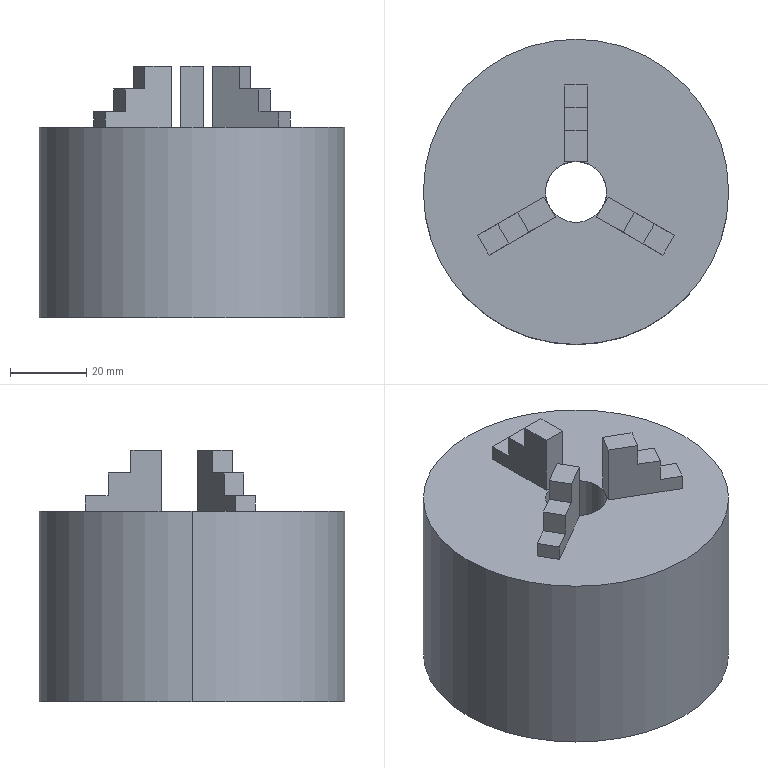Part | SolidWorks | features ICE 4, CirPattern 2, Extrusion 1, HoleWzd 1 | 1 solid | 45 faces | box 80 x 80 x 66 mm | volume 244059 mm3 | plane 29 | cylinder 10 | cone 6 | commonest cylinder face diameters 5 x6 16 x2 80 x2
STEP:
#1=CARTESIAN_POINT('',(-26.079,-16.5,17.));
#2=VERTEX_POINT('',#1);
#3=CARTESIAN_POINT('',(-31.079,-16.5,17.));
#4=VERTEX_POINT('',#3);
#5=CARTESIAN_POINT('',(-28.579,-16.5,17.));
#6=DIRECTION('',(0.,0.,-1.));
#7=DIRECTION('',(-1.,0.,0.));
#8=AXIS2_PLACEMENT_3D('',#5,#6,#7);
#9=CIRCLE('',#8,2.5);
#10=EDGE_CURVE('',#2,#4,#9,.T.);
#11=ORIENTED_EDGE('',*,*,#10,.F.);
#12=CARTESIAN_POINT('',(-26.079,-16.5,0.));
#13=VERTEX_POINT('',#12);
#14=CARTESIAN_POINT('',(-26.079,-16.5,0.));
#15=DIRECTION('',(0.,0.,-1.));
#16=VECTOR('',#15,1000.);
#17=LINE('',#14,#16);
#18=EDGE_CURVE('',#2,#13,#17,.T.);
#19=ORIENTED_EDGE('',*,*,#18,.T.);
#20=CARTESIAN_POINT('',(-31.079,-16.5,0.));
#21=VERTEX_POINT('',#20);
#22=CARTESIAN_POINT('',(-28.579,-16.5,0.));
#23=DIRECTION('',(0.,0.,-1.));
#24=DIRECTION('',(-1.,0.,0.));
#25=AXIS2_PLACEMENT_3D('',#22,#23,#24);
#26=CIRCLE('',#25,2.5);
#27=EDGE_CURVE('',#13,#21,#26,.T.);
#28=ORIENTED_EDGE('',*,*,#27,.T.);
#29=CARTESIAN_POINT('',(-31.079,-16.5,0.));
#30=DIRECTION('',(0.,0.,-1.));
#31=VECTOR('',#30,1000.);
#32=LINE('',#29,#31);
#33=EDGE_CURVE('',#4,#21,#32,.T.);
#34=ORIENTED_EDGE('',*,*,#33,.F.);
#35=EDGE_LOOP('',(#11,#19,#28,#34));
#36=FACE_OUTER_BOUND('',#35,.T.);
#37=CARTESIAN_POINT('',(-28.579,-16.5,0.));
#38=DIRECTION('',(0.,0.,-1.));
#39=DIRECTION('',(-1.,0.,0.));
#40=AXIS2_PLACEMENT_3D('',#37,#38,#39);
#41=CYLINDRICAL_SURFACE('',#40,2.5);
#42=ADVANCED_FACE('',(#36),#41,.F.);
#43=CARTESIAN_POINT('',(-28.579,-16.5,18.502));
#44=VERTEX_POINT('',#43);
#45=CARTESIAN_POINT('',(-31.079,-16.5,17.));
#46=DIRECTION('',(-0.8572,0.,-0.515));
#47=VECTOR('',#46,1000.);
#48=LINE('',#45,#47);
#49=EDGE_CURVE('',#44,#4,#48,.T.);
#50=ORIENTED_EDGE('',*,*,#49,.F.);
#51=CARTESIAN_POINT('',(-26.079,-16.5,17.));
#52=DIRECTION('',(0.8572,0.,-0.515));
#53=VECTOR('',#52,1000.);
#54=LINE('',#51,#53);
#55=EDGE_CURVE('',#44,#2,#54,.T.);
#56=ORIENTED_EDGE('',*,*,#55,.T.);
#57=ORIENTED_EDGE('',*,*,#10,.T.);
#58=EDGE_LOOP('',(#50,#56,#57));
#59=FACE_OUTER_BOUND('',#58,.T.);
#60=CARTESIAN_POINT('',(-28.579,-16.5,17.));
#61=DIRECTION('',(0.,0.,-1.));
#62=DIRECTION('',(-1.,0.,0.));
#63=AXIS2_PLACEMENT_3D('',#60,#61,#62);
#64=CONICAL_SURFACE('',#63,2.5,1.03);
#65=ADVANCED_FACE('',(#59),#64,.F.);
#66=CARTESIAN_POINT('',(31.079,-16.5,17.));
#67=VERTEX_POINT('',#66);
#68=CARTESIAN_POINT('',(26.079,-16.5,17.));
#69=VERTEX_POINT('',#68);
#70=CARTESIAN_POINT('',(28.579,-16.5,17.));
#71=DIRECTION('',(0.,0.,-1.));
#72=DIRECTION('',(-1.,0.,0.));
#73=AXIS2_PLACEMENT_3D('',#70,#71,#72);
#74=CIRCLE('',#73,2.5);
#75=EDGE_CURVE('',#67,#69,#74,.T.);
#76=ORIENTED_EDGE('',*,*,#75,.F.);
#77=CARTESIAN_POINT('',(31.079,-16.5,0.));
#78=VERTEX_POINT('',#77);
#79=CARTESIAN_POINT('',(31.079,-16.5,0.));
#80=DIRECTION('',(0.,0.,-1.));
#81=VECTOR('',#80,1000.);
#82=LINE('',#79,#81);
#83=EDGE_CURVE('',#67,#78,#82,.T.);
#84=ORIENTED_EDGE('',*,*,#83,.T.);
#85=CARTESIAN_POINT('',(26.079,-16.5,0.));
#86=VERTEX_POINT('',#85);
#87=CARTESIAN_POINT('',(28.579,-16.5,0.));
#88=DIRECTION('',(0.,0.,-1.));
#89=DIRECTION('',(-1.,0.,0.));
#90=AXIS2_PLACEMENT_3D('',#87,#88,#89);
#91=CIRCLE('',#90,2.5);
#92=EDGE_CURVE('',#78,#86,#91,.T.);
#93=ORIENTED_EDGE('',*,*,#92,.T.);
#94=CARTESIAN_POINT('',(26.079,-16.5,0.));
#95=DIRECTION('',(0.,0.,-1.));
#96=VECTOR('',#95,1000.);
#97=LINE('',#94,#96);
#98=EDGE_CURVE('',#69,#86,#97,.T.);
#99=ORIENTED_EDGE('',*,*,#98,.F.);
#100=EDGE_LOOP('',(#76,#84,#93,#99));
#101=FACE_OUTER_BOUND('',#100,.T.);
#102=CARTESIAN_POINT('',(28.579,-16.5,0.));
#103=DIRECTION('',(0.,0.,-1.));
#104=DIRECTION('',(-1.,0.,0.));
#105=AXIS2_PLACEMENT_3D('',#102,#103,#104);
#106=CYLINDRICAL_SURFACE('',#105,2.5);
#107=ADVANCED_FACE('',(#101),#106,.F.);
#108=CARTESIAN_POINT('',(28.579,-16.5,18.502));
#109=VERTEX_POINT('',#108);
#110=CARTESIAN_POINT('',(26.079,-16.5,17.));
#111=DIRECTION('',(-0.8572,0.,-0.515));
#112=VECTOR('',#111,1000.);
#113=LINE('',#110,#112);
#114=EDGE_CURVE('',#109,#69,#113,.T.);
#115=ORIENTED_EDGE('',*,*,#114,.F.);
#116=CARTESIAN_POINT('',(31.079,-16.5,17.));
#117=DIRECTION('',(0.8572,0.,-0.515));
#118=VECTOR('',#117,1000.);
#119=LINE('',#116,#118);
#120=EDGE_CURVE('',#109,#67,#119,.T.);
#121=ORIENTED_EDGE('',*,*,#120,.T.);
#122=ORIENTED_EDGE('',*,*,#75,.T.);
#123=EDGE_LOOP('',(#115,#121,#122));
#124=FACE_OUTER_BOUND('',#123,.T.);
#125=CARTESIAN_POINT('',(28.579,-16.5,17.));
#126=DIRECTION('',(0.,0.,-1.));
#127=DIRECTION('',(-1.,0.,0.));
#128=AXIS2_PLACEMENT_3D('',#125,#126,#127);
#129=CONICAL_SURFACE('',#128,2.5,1.03);
#130=ADVANCED_FACE('',(#124),#129,.F.);
#131=CARTESIAN_POINT('',(2.5,33.,17.));
#132=VERTEX_POINT('',#131);
#133=CARTESIAN_POINT('',(-2.5,33.,17.));
#134=VERTEX_POINT('',#133);
#135=CARTESIAN_POINT('',(0.,33.,17.));
#136=DIRECTION('',(0.,0.,-1.));
#137=DIRECTION('',(-1.,0.,0.));
#138=AXIS2_PLACEMENT_3D('',#135,#136,#137);
#139=CIRCLE('',#138,2.5);
#140=EDGE_CURVE('',#132,#134,#139,.T.);
#141=ORIENTED_EDGE('',*,*,#140,.F.);
#142=CARTESIAN_POINT('',(2.5,33.,0.));
#143=VERTEX_POINT('',#142);
#144=CARTESIAN_POINT('',(2.5,33.,0.));
#145=DIRECTION('',(0.,0.,-1.));
#146=VECTOR('',#145,1000.);
#147=LINE('',#144,#146);
#148=EDGE_CURVE('',#132,#143,#147,.T.);
#149=ORIENTED_EDGE('',*,*,#148,.T.);
#150=CARTESIAN_POINT('',(-2.5,33.,0.));
#151=VERTEX_POINT('',#150);
#152=CARTESIAN_POINT('',(0.,33.,0.));
#153=DIRECTION('',(0.,0.,-1.));
#154=DIRECTION('',(-1.,0.,0.));
#155=AXIS2_PLACEMENT_3D('',#152,#153,#154);
#156=CIRCLE('',#155,2.5);
#157=EDGE_CURVE('',#143,#151,#156,.T.);
#158=ORIENTED_EDGE('',*,*,#157,.T.);
#159=CARTESIAN_POINT('',(-2.5,33.,0.));
#160=DIRECTION('',(0.,0.,-1.));
#161=VECTOR('',#160,1000.);
#162=LINE('',#159,#161);
#163=EDGE_CURVE('',#134,#151,#162,.T.);
#164=ORIENTED_EDGE('',*,*,#163,.F.);
#165=EDGE_LOOP('',(#141,#149,#158,#164));
#166=FACE_OUTER_BOUND('',#165,.T.);
#167=CARTESIAN_POINT('',(0.,33.,0.));
#168=DIRECTION('',(0.,0.,-1.));
#169=DIRECTION('',(-1.,0.,0.));
#170=AXIS2_PLACEMENT_3D('',#167,#168,#169);
#171=CYLINDRICAL_SURFACE('',#170,2.5);
#172=ADVANCED_FACE('',(#166),#171,.F.);
#173=CARTESIAN_POINT('',(0.,33.,18.502));
#174=VERTEX_POINT('',#173);
#175=CARTESIAN_POINT('',(-2.5,33.,17.));
#176=DIRECTION('',(-0.8572,0.,-0.515));
#177=VECTOR('',#176,1000.);
#178=LINE('',#175,#177);
#179=EDGE_CURVE('',#174,#134,#178,.T.);
#180=ORIENTED_EDGE('',*,*,#179,.F.);
#181=CARTESIAN_POINT('',(2.5,33.,17.));
#182=DIRECTION('',(0.8572,0.,-0.515));
#183=VECTOR('',#182,1000.);
#184=LINE('',#181,#183);
#185=EDGE_CURVE('',#174,#132,#184,.T.);
#186=ORIENTED_EDGE('',*,*,#185,.T.);
#187=ORIENTED_EDGE('',*,*,#140,.T.);
#188=EDGE_LOOP('',(#180,#186,#187));
#189=FACE_OUTER_BOUND('',#188,.T.);
#190=CARTESIAN_POINT('',(0.,33.,17.));
#191=DIRECTION('',(0.,0.,-1.));
#192=DIRECTION('',(-1.,0.,0.));
#193=AXIS2_PLACEMENT_3D('',#190,#191,#192);
#194=CONICAL_SURFACE('',#193,2.5,1.03);
#195=ADVANCED_FACE('',(#189),#194,.F.);
#196=CARTESIAN_POINT('',(6.928,-4.,50.));
#197=VERTEX_POINT('',#196);
#198=CARTESIAN_POINT('',(8.,0.,50.));
#199=VERTEX_POINT('',#198);
#200=CARTESIAN_POINT('',(0.,0.,50.));
#201=DIRECTION('',(0.,0.,1.));
#202=DIRECTION('',(1.,0.,0.));
#203=AXIS2_PLACEMENT_3D('',#200,#201,#202);
#204=CIRCLE('',#203,8.);
#205=EDGE_CURVE('',#197,#199,#204,.T.);
#206=ORIENTED_EDGE('',*,*,#205,.T.);
#207=CARTESIAN_POINT('',(8.,0.,0.));
#208=VERTEX_POINT('',#207);
#209=CARTESIAN_POINT('',(8.,0.,66.));
#210=DIRECTION('',(0.,0.,-1.));
#211=VECTOR('',#210,1000.);
#212=LINE('',#209,#211);
#213=EDGE_CURVE('',#199,#208,#212,.T.);
#214=ORIENTED_EDGE('',*,*,#213,.T.);
#215=CARTESIAN_POINT('',(-8.,0.,0.));
#216=VERTEX_POINT('',#215);
#217=CARTESIAN_POINT('',(0.,0.,0.));
#218=DIRECTION('',(0.,0.,-1.));
#219=DIRECTION('',(-1.,0.,0.));
#220=AXIS2_PLACEMENT_3D('',#217,#218,#219);
#221=CIRCLE('',#220,8.);
#222=EDGE_CURVE('',#208,#216,#221,.T.);
#223=ORIENTED_EDGE('',*,*,#222,.T.);
#224=CARTESIAN_POINT('',(-8.,0.,50.));
#225=VERTEX_POINT('',#224);
#226=CARTESIAN_POINT('',(-8.,0.,66.));
#227=DIRECTION('',(0.,0.,-1.));
#228=VECTOR('',#227,1000.);
#229=LINE('',#226,#228);
#230=EDGE_CURVE('',#225,#216,#229,.T.);
#231=ORIENTED_EDGE('',*,*,#230,.F.);
#232=CARTESIAN_POINT('',(-6.928,-4.,50.));
#233=VERTEX_POINT('',#232);
#234=CARTESIAN_POINT('',(0.,0.,50.));
#235=DIRECTION('',(0.,0.,1.));
#236=DIRECTION('',(1.,0.,0.));
#237=AXIS2_PLACEMENT_3D('',#234,#235,#236);
#238=CIRCLE('',#237,8.);
#239=EDGE_CURVE('',#225,#233,#238,.T.);
#240=ORIENTED_EDGE('',*,*,#239,.T.);
#241=CARTESIAN_POINT('',(0.,0.,50.));
#242=DIRECTION('',(0.,0.,1.));
#243=DIRECTION('',(1.,0.,0.));
#244=AXIS2_PLACEMENT_3D('',#241,#242,#243);
#245=CIRCLE('',#244,8.);
#246=EDGE_CURVE('',#233,#197,#245,.T.);
#247=ORIENTED_EDGE('',*,*,#246,.T.);
#248=EDGE_LOOP('',(#206,#214,#223,#231,#240,#247));
#249=FACE_OUTER_BOUND('',#248,.T.);
#250=CARTESIAN_POINT('',(0.,0.,66.));
#251=DIRECTION('',(0.,0.,-1.));
#252=DIRECTION('',(-1.,0.,0.));
#253=AXIS2_PLACEMENT_3D('',#250,#251,#252);
#254=CYLINDRICAL_SURFACE('',#253,8.);
#255=ADVANCED_FACE('',(#249),#254,.F.);
#256=CARTESIAN_POINT('',(40.,0.,50.));
#257=VERTEX_POINT('',#256);
#258=CARTESIAN_POINT('',(-40.,0.,50.));
#259=VERTEX_POINT('',#258);
#260=CARTESIAN_POINT('',(0.,0.,50.));
#261=DIRECTION('',(0.,0.,1.));
#262=DIRECTION('',(1.,0.,0.));
#263=AXIS2_PLACEMENT_3D('',#260,#261,#262);
#264=CIRCLE('',#263,40.);
#265=EDGE_CURVE('',#257,#259,#264,.T.);
#266=ORIENTED_EDGE('',*,*,#265,.F.);
#267=CARTESIAN_POINT('',(40.,0.,0.));
#268=VERTEX_POINT('',#267);
#269=CARTESIAN_POINT('',(40.,0.,50.));
#270=DIRECTION('',(0.,0.,-1.));
#271=VECTOR('',#270,1000.);
#272=LINE('',#269,#271);
#273=EDGE_CURVE('',#257,#268,#272,.T.);
#274=ORIENTED_EDGE('',*,*,#273,.T.);
#275=CARTESIAN_POINT('',(-40.,0.,0.));
#276=VERTEX_POINT('',#275);
#277=CARTESIAN_POINT('',(0.,0.,0.));
#278=DIRECTION('',(0.,0.,1.));
#279=DIRECTION('',(1.,0.,0.));
#280=AXIS2_PLACEMENT_3D('',#277,#278,#279);
#281=CIRCLE('',#280,40.);
#282=EDGE_CURVE('',#268,#276,#281,.T.);
#283=ORIENTED_EDGE('',*,*,#282,.T.);
#284=CARTESIAN_POINT('',(-40.,0.,50.));
#285=DIRECTION('',(0.,0.,-1.));
#286=VECTOR('',#285,1000.);
#287=LINE('',#284,#286);
#288=EDGE_CURVE('',#259,#276,#287,.T.);
#289=ORIENTED_EDGE('',*,*,#288,.F.);
#290=EDGE_LOOP('',(#266,#274,#283,#289));
#291=FACE_OUTER_BOUND('',#290,.T.);
#292=CARTESIAN_POINT('',(0.,0.,50.));
#293=DIRECTION('',(0.,0.,-1.));
#294=DIRECTION('',(-1.,0.,0.));
#295=AXIS2_PLACEMENT_3D('',#292,#293,#294);
#296=CYLINDRICAL_SURFACE('',#295,40.);
#297=ADVANCED_FACE('',(#291),#296,.T.);
#298=CARTESIAN_POINT('',(0.,8.,50.));
#299=VERTEX_POINT('',#298);
#300=CARTESIAN_POINT('',(0.,0.,50.));
#301=DIRECTION('',(0.,0.,1.));
#302=DIRECTION('',(1.,0.,0.));
#303=AXIS2_PLACEMENT_3D('',#300,#301,#302);
#304=CIRCLE('',#303,8.);
#305=EDGE_CURVE('',#299,#225,#304,.T.);
#306=ORIENTED_EDGE('',*,*,#305,.F.);
#307=CARTESIAN_POINT('',(-3.,8.,50.));
#308=VERTEX_POINT('',#307);
#309=CARTESIAN_POINT('',(-3.,8.,50.));
#310=DIRECTION('',(1.,0.,0.));
#311=VECTOR('',#310,1000.);
#312=LINE('',#309,#311);
#313=EDGE_CURVE('',#308,#299,#312,.T.);
#314=ORIENTED_EDGE('',*,*,#313,.F.);
#315=CARTESIAN_POINT('',(-3.,28.,50.));
#316=VERTEX_POINT('',#315);
#317=CARTESIAN_POINT('',(-3.,8.,50.));
#318=DIRECTION('',(0.,-1.,0.));
#319=VECTOR('',#318,1000.);
#320=LINE('',#317,#319);
#321=EDGE_CURVE('',#316,#308,#320,.T.);
#322=ORIENTED_EDGE('',*,*,#321,.F.);
#323=CARTESIAN_POINT('',(3.,28.,50.));
#324=VERTEX_POINT('',#323);
#325=CARTESIAN_POINT('',(-3.,28.,50.));
#326=DIRECTION('',(-1.,0.,0.));
#327=VECTOR('',#326,1000.);
#328=LINE('',#325,#327);
#329=EDGE_CURVE('',#324,#316,#328,.T.);
#330=ORIENTED_EDGE('',*,*,#329,.F.);
#331=CARTESIAN_POINT('',(3.,8.,50.));
#332=VERTEX_POINT('',#331);
#333=CARTESIAN_POINT('',(3.,8.,50.));
#334=DIRECTION('',(0.,1.,0.));
#335=VECTOR('',#334,1000.);
#336=LINE('',#333,#335);
#337=EDGE_CURVE('',#332,#324,#336,.T.);
#338=ORIENTED_EDGE('',*,*,#337,.F.);
#339=CARTESIAN_POINT('',(-3.,8.,50.));
#340=DIRECTION('',(1.,0.,0.));
#341=VECTOR('',#340,1000.);
#342=LINE('',#339,#341);
#343=EDGE_CURVE('',#299,#332,#342,.T.);
#344=ORIENTED_EDGE('',*,*,#343,.F.);
#345=CARTESIAN_POINT('',(0.,0.,50.));
#346=DIRECTION('',(0.,0.,1.));
#347=DIRECTION('',(1.,0.,0.));
#348=AXIS2_PLACEMENT_3D('',#345,#346,#347);
#349=CIRCLE('',#348,8.);
#350=EDGE_CURVE('',#199,#299,#349,.T.);
#351=ORIENTED_EDGE('',*,*,#350,.F.);
#352=ORIENTED_EDGE('',*,*,#205,.F.);
#353=CARTESIAN_POINT('',(8.428,-1.402,50.));
#354=VERTEX_POINT('',#353);
#355=CARTESIAN_POINT('',(8.428,-1.402,50.));
#356=DIRECTION('',(-0.5,-0.866,0.));
#357=VECTOR('',#356,1000.);
#358=LINE('',#355,#357);
#359=EDGE_CURVE('',#354,#197,#358,.T.);
#360=ORIENTED_EDGE('',*,*,#359,.F.);
#361=CARTESIAN_POINT('',(25.749,-11.402,50.));
#362=VERTEX_POINT('',#361);
#363=CARTESIAN_POINT('',(8.428,-1.402,50.));
#364=DIRECTION('',(-0.866,0.5,0.));
#365=VECTOR('',#364,1000.);
#366=LINE('',#363,#365);
#367=EDGE_CURVE('',#362,#354,#366,.T.);
#368=ORIENTED_EDGE('',*,*,#367,.F.);
#369=CARTESIAN_POINT('',(22.749,-16.598,50.));
#370=VERTEX_POINT('',#369);
#371=CARTESIAN_POINT('',(25.749,-11.402,50.));
#372=DIRECTION('',(0.5,0.866,0.));
#373=VECTOR('',#372,1000.);
#374=LINE('',#371,#373);
#375=EDGE_CURVE('',#370,#362,#374,.T.);
#376=ORIENTED_EDGE('',*,*,#375,.F.);
#377=CARTESIAN_POINT('',(5.428,-6.598,50.));
#378=VERTEX_POINT('',#377);
#379=CARTESIAN_POINT('',(5.428,-6.598,50.));
#380=DIRECTION('',(0.866,-0.5,0.));
#381=VECTOR('',#380,1000.);
#382=LINE('',#379,#381);
#383=EDGE_CURVE('',#378,#370,#382,.T.);
#384=ORIENTED_EDGE('',*,*,#383,.F.);
#385=CARTESIAN_POINT('',(8.428,-1.402,50.));
#386=DIRECTION('',(-0.5,-0.866,0.));
#387=VECTOR('',#386,1000.);
#388=LINE('',#385,#387);
#389=EDGE_CURVE('',#197,#378,#388,.T.);
#390=ORIENTED_EDGE('',*,*,#389,.F.);
#391=ORIENTED_EDGE('',*,*,#246,.F.);
#392=CARTESIAN_POINT('',(-5.428,-6.598,50.));
#393=VERTEX_POINT('',#392);
#394=CARTESIAN_POINT('',(-5.428,-6.598,50.));
#395=DIRECTION('',(-0.5,0.866,0.));
#396=VECTOR('',#395,1000.);
#397=LINE('',#394,#396);
#398=EDGE_CURVE('',#393,#233,#397,.T.);
#399=ORIENTED_EDGE('',*,*,#398,.F.);
#400=CARTESIAN_POINT('',(-22.749,-16.598,50.));
#401=VERTEX_POINT('',#400);
#402=CARTESIAN_POINT('',(-5.428,-6.598,50.));
#403=DIRECTION('',(0.866,0.5,0.));
#404=VECTOR('',#403,1000.);
#405=LINE('',#402,#404);
#406=EDGE_CURVE('',#401,#393,#405,.T.);
#407=ORIENTED_EDGE('',*,*,#406,.F.);
#408=CARTESIAN_POINT('',(-25.749,-11.402,50.));
#409=VERTEX_POINT('',#408);
#410=CARTESIAN_POINT('',(-22.749,-16.598,50.));
#411=DIRECTION('',(0.5,-0.866,0.));
#412=VECTOR('',#411,1000.);
#413=LINE('',#410,#412);
#414=EDGE_CURVE('',#409,#401,#413,.T.);
#415=ORIENTED_EDGE('',*,*,#414,.F.);
#416=CARTESIAN_POINT('',(-8.428,-1.402,50.));
#417=VERTEX_POINT('',#416);
#418=CARTESIAN_POINT('',(-8.428,-1.402,50.));
#419=DIRECTION('',(-0.866,-0.5,0.));
#420=VECTOR('',#419,1000.);
#421=LINE('',#418,#420);
#422=EDGE_CURVE('',#417,#409,#421,.T.);
#423=ORIENTED_EDGE('',*,*,#422,.F.);
#424=CARTESIAN_POINT('',(-5.428,-6.598,50.));
#425=DIRECTION('',(-0.5,0.866,0.));
#426=VECTOR('',#425,1000.);
#427=LINE('',#424,#426);
#428=EDGE_CURVE('',#233,#417,#427,.T.);
#429=ORIENTED_EDGE('',*,*,#428,.F.);
#430=ORIENTED_EDGE('',*,*,#239,.F.);
#431=EDGE_LOOP('',(#306,#314,#322,#330,#338,#344,#351,#352,#360,#368,#376,#384,#390,#391,#399,#407,#415,#423,#429,#430));
#432=FACE_BOUND('',#431,.T.);
#433=CARTESIAN_POINT('',(0.,0.,50.));
#434=DIRECTION('',(0.,0.,1.));
#435=DIRECTION('',(1.,0.,0.));
#436=AXIS2_PLACEMENT_3D('',#433,#434,#435);
#437=CIRCLE('',#436,40.);
#438=EDGE_CURVE('',#259,#257,#437,.T.);
#439=ORIENTED_EDGE('',*,*,#438,.T.);
#440=ORIENTED_EDGE('',*,*,#265,.T.);
#441=EDGE_LOOP('',(#439,#440));
#442=FACE_OUTER_BOUND('',#441,.T.);
#443=CARTESIAN_POINT('',(0.,0.,50.));
#444=DIRECTION('',(0.,0.,1.));
#445=DIRECTION('',(1.,0.,0.));
#446=AXIS2_PLACEMENT_3D('',#443,#444,#445);
#447=PLANE('',#446);
#448=ADVANCED_FACE('',(#432,#442),#447,.T.);
#449=ORIENTED_EDGE('',*,*,#273,.F.);
#450=ORIENTED_EDGE('',*,*,#438,.F.);
#451=ORIENTED_EDGE('',*,*,#288,.T.);
#452=CARTESIAN_POINT('',(0.,0.,0.));
#453=DIRECTION('',(0.,0.,1.));
#454=DIRECTION('',(1.,0.,0.));
#455=AXIS2_PLACEMENT_3D('',#452,#453,#454);
#456=CIRCLE('',#455,40.);
#457=EDGE_CURVE('',#276,#268,#456,.T.);
#458=ORIENTED_EDGE('',*,*,#457,.T.);
#459=EDGE_LOOP('',(#449,#450,#451,#458));
#460=FACE_OUTER_BOUND('',#459,.T.);
#461=CARTESIAN_POINT('',(0.,0.,50.));
#462=DIRECTION('',(0.,0.,-1.));
#463=DIRECTION('',(-1.,0.,0.));
#464=AXIS2_PLACEMENT_3D('',#461,#462,#463);
#465=CYLINDRICAL_SURFACE('',#464,40.);
#466=ADVANCED_FACE('',(#460),#465,.T.);
#467=CARTESIAN_POINT('',(-28.579,-16.5,0.));
#468=DIRECTION('',(0.,0.,-1.));
#469=DIRECTION('',(-1.,0.,0.));
#470=AXIS2_PLACEMENT_3D('',#467,#468,#469);
#471=CIRCLE('',#470,2.5);
#472=EDGE_CURVE('',#21,#13,#471,.T.);
#473=ORIENTED_EDGE('',*,*,#472,.F.);
#474=ORIENTED_EDGE('',*,*,#27,.F.);
#475=EDGE_LOOP('',(#473,#474));
#476=FACE_BOUND('',#475,.T.);
#477=CARTESIAN_POINT('',(28.579,-16.5,0.));
#478=DIRECTION('',(0.,0.,-1.));
#479=DIRECTION('',(-1.,0.,0.));
#480=AXIS2_PLACEMENT_3D('',#477,#478,#479);
#481=CIRCLE('',#480,2.5);
#482=EDGE_CURVE('',#86,#78,#481,.T.);
#483=ORIENTED_EDGE('',*,*,#482,.F.);
#484=ORIENTED_EDGE('',*,*,#92,.F.);
#485=EDGE_LOOP('',(#483,#484));
#486=FACE_BOUND('',#485,.T.);
#487=CARTESIAN_POINT('',(0.,33.,0.));
#488=DIRECTION('',(0.,0.,-1.));
#489=DIRECTION('',(-1.,0.,0.));
#490=AXIS2_PLACEMENT_3D('',#487,#488,#489);
#491=CIRCLE('',#490,2.5);
#492=EDGE_CURVE('',#151,#143,#491,.T.);
#493=ORIENTED_EDGE('',*,*,#492,.F.);
#494=ORIENTED_EDGE('',*,*,#157,.F.);
#495=EDGE_LOOP('',(#493,#494));
#496=FACE_BOUND('',#495,.T.);
#497=CARTESIAN_POINT('',(0.,0.,0.));
#498=DIRECTION('',(0.,0.,-1.));
#499=DIRECTION('',(-1.,0.,0.));
#500=AXIS2_PLACEMENT_3D('',#497,#498,#499);
#501=CIRCLE('',#500,8.);
#502=EDGE_CURVE('',#216,#208,#501,.T.);
#503=ORIENTED_EDGE('',*,*,#502,.F.);
#504=ORIENTED_EDGE('',*,*,#222,.F.);
#505=EDGE_LOOP('',(#503,#504));
#506=FACE_BOUND('',#505,.T.);
#507=ORIENTED_EDGE('',*,*,#457,.F.);
#508=ORIENTED_EDGE('',*,*,#282,.F.);
#509=EDGE_LOOP('',(#507,#508));
#510=FACE_OUTER_BOUND('',#509,.T.);
#511=CARTESIAN_POINT('',(0.,0.,0.));
#512=DIRECTION('',(0.,0.,1.));
#513=DIRECTION('',(1.,0.,0.));
#514=AXIS2_PLACEMENT_3D('',#511,#512,#513);
#515=PLANE('',#514);
#516=ADVANCED_FACE('',(#476,#486,#496,#506,#510),#515,.F.);
#517=CARTESIAN_POINT('',(3.,22.,60.));
#518=VERTEX_POINT('',#517);
#519=CARTESIAN_POINT('',(3.,16.,60.));
#520=VERTEX_POINT('',#519);
#521=CARTESIAN_POINT('',(3.,8.,60.));
#522=DIRECTION('',(0.,-1.,0.));
#523=VECTOR('',#522,1000.);
#524=LINE('',#521,#523);
#525=EDGE_CURVE('',#518,#520,#524,.T.);
#526=ORIENTED_EDGE('',*,*,#525,.T.);
#527=CARTESIAN_POINT('',(3.,16.,66.));
#528=VERTEX_POINT('',#527);
#529=CARTESIAN_POINT('',(3.,16.,66.));
#530=DIRECTION('',(0.,0.,1.));
#531=VECTOR('',#530,1000.);
#532=LINE('',#529,#531);
#533=EDGE_CURVE('',#520,#528,#532,.T.);
#534=ORIENTED_EDGE('',*,*,#533,.T.);
#535=CARTESIAN_POINT('',(3.,8.,66.));
#536=VERTEX_POINT('',#535);
#537=CARTESIAN_POINT('',(3.,8.,66.));
#538=DIRECTION('',(0.,1.,0.));
#539=VECTOR('',#538,1000.);
#540=LINE('',#537,#539);
#541=EDGE_CURVE('',#536,#528,#540,.T.);
#542=ORIENTED_EDGE('',*,*,#541,.F.);
#543=CARTESIAN_POINT('',(3.,8.,66.));
#544=DIRECTION('',(0.,0.,-1.));
#545=VECTOR('',#544,1000.);
#546=LINE('',#543,#545);
#547=EDGE_CURVE('',#536,#332,#546,.T.);
#548=ORIENTED_EDGE('',*,*,#547,.T.);
#549=ORIENTED_EDGE('',*,*,#337,.T.);
#550=CARTESIAN_POINT('',(3.,28.,54.));
#551=VERTEX_POINT('',#550);
#552=CARTESIAN_POINT('',(3.,28.,66.));
#553=DIRECTION('',(0.,0.,-1.));
#554=VECTOR('',#553,1000.);
#555=LINE('',#552,#554);
#556=EDGE_CURVE('',#551,#324,#555,.T.);
#557=ORIENTED_EDGE('',*,*,#556,.F.);
#558=CARTESIAN_POINT('',(3.,22.,54.));
#559=VERTEX_POINT('',#558);
#560=CARTESIAN_POINT('',(3.,8.,54.));
#561=DIRECTION('',(0.,-1.,0.));
#562=VECTOR('',#561,1000.);
#563=LINE('',#560,#562);
#564=EDGE_CURVE('',#551,#559,#563,.T.);
#565=ORIENTED_EDGE('',*,*,#564,.T.);
#566=CARTESIAN_POINT('',(3.,22.,66.));
#567=DIRECTION('',(0.,0.,1.));
#568=VECTOR('',#567,1000.);
#569=LINE('',#566,#568);
#570=EDGE_CURVE('',#559,#518,#569,.T.);
#571=ORIENTED_EDGE('',*,*,#570,.T.);
#572=EDGE_LOOP('',(#526,#534,#542,#548,#549,#557,#565,#571));
#573=FACE_OUTER_BOUND('',#572,.T.);
#574=CARTESIAN_POINT('',(3.,8.,66.));
#575=DIRECTION('',(-1.,0.,0.));
#576=DIRECTION('',(0.,0.,1.));
#577=AXIS2_PLACEMENT_3D('',#574,#575,#576);
#578=PLANE('',#577);
#579=ADVANCED_FACE('',(#573),#578,.F.);
#580=CARTESIAN_POINT('',(-3.,28.,54.));
#581=VERTEX_POINT('',#580);
#582=CARTESIAN_POINT('',(-3.,28.,66.));
#583=DIRECTION('',(0.,0.,-1.));
#584=VECTOR('',#583,1000.);
#585=LINE('',#582,#584);
#586=EDGE_CURVE('',#581,#316,#585,.T.);
#587=ORIENTED_EDGE('',*,*,#586,.F.);
#588=CARTESIAN_POINT('',(40.,28.,54.));
#589=DIRECTION('',(-1.,0.,0.));
#590=VECTOR('',#589,1000.);
#591=LINE('',#588,#590);
#592=EDGE_CURVE('',#551,#581,#591,.T.);
#593=ORIENTED_EDGE('',*,*,#592,.F.);
#594=ORIENTED_EDGE('',*,*,#556,.T.);
#595=ORIENTED_EDGE('',*,*,#329,.T.);
#596=EDGE_LOOP('',(#587,#593,#594,#595));
#597=FACE_OUTER_BOUND('',#596,.T.);
#598=CARTESIAN_POINT('',(-3.,28.,66.));
#599=DIRECTION('',(0.,-1.,0.));
#600=DIRECTION('',(0.,0.,-1.));
#601=AXIS2_PLACEMENT_3D('',#598,#599,#600);
#602=PLANE('',#601);
#603=ADVANCED_FACE('',(#597),#602,.F.);
#604=CARTESIAN_POINT('',(-3.,16.,66.));
#605=VERTEX_POINT('',#604);
#606=CARTESIAN_POINT('',(-3.,8.,66.));
#607=VERTEX_POINT('',#606);
#608=CARTESIAN_POINT('',(-3.,8.,66.));
#609=DIRECTION('',(0.,-1.,0.));
#610=VECTOR('',#609,1000.);
#611=LINE('',#608,#610);
#612=EDGE_CURVE('',#605,#607,#611,.T.);
#613=ORIENTED_EDGE('',*,*,#612,.F.);
#614=CARTESIAN_POINT('',(-3.,16.,60.));
#615=VERTEX_POINT('',#614);
#616=CARTESIAN_POINT('',(-3.,16.,60.));
#617=DIRECTION('',(0.,0.,1.));
#618=VECTOR('',#617,1000.);
#619=LINE('',#616,#618);
#620=EDGE_CURVE('',#615,#605,#619,.T.);
#621=ORIENTED_EDGE('',*,*,#620,.F.);
#622=CARTESIAN_POINT('',(-3.,22.,60.));
#623=VERTEX_POINT('',#622);
#624=CARTESIAN_POINT('',(-3.,22.,60.));
#625=DIRECTION('',(0.,-1.,0.));
#626=VECTOR('',#625,1000.);
#627=LINE('',#624,#626);
#628=EDGE_CURVE('',#623,#615,#627,.T.);
#629=ORIENTED_EDGE('',*,*,#628,.F.);
#630=CARTESIAN_POINT('',(-3.,22.,54.));
#631=VERTEX_POINT('',#630);
#632=CARTESIAN_POINT('',(-3.,22.,54.));
#633=DIRECTION('',(0.,0.,1.));
#634=VECTOR('',#633,1000.);
#635=LINE('',#632,#634);
#636=EDGE_CURVE('',#631,#623,#635,.T.);
#637=ORIENTED_EDGE('',*,*,#636,.F.);
#638=CARTESIAN_POINT('',(-3.,28.,54.));
#639=DIRECTION('',(0.,-1.,0.));
#640=VECTOR('',#639,1000.);
#641=LINE('',#638,#640);
#642=EDGE_CURVE('',#581,#631,#641,.T.);
#643=ORIENTED_EDGE('',*,*,#642,.F.);
#644=ORIENTED_EDGE('',*,*,#586,.T.);
#645=ORIENTED_EDGE('',*,*,#321,.T.);
#646=CARTESIAN_POINT('',(-3.,8.,66.));
#647=DIRECTION('',(0.,0.,-1.));
#648=VECTOR('',#647,1000.);
#649=LINE('',#646,#648);
#650=EDGE_CURVE('',#607,#308,#649,.T.);
#651=ORIENTED_EDGE('',*,*,#650,.F.);
#652=EDGE_LOOP('',(#613,#621,#629,#637,#643,#644,#645,#651));
#653=FACE_OUTER_BOUND('',#652,.T.);
#654=CARTESIAN_POINT('',(-3.,8.,66.));
#655=DIRECTION('',(1.,0.,0.));
#656=DIRECTION('',(0.,0.,-1.));
#657=AXIS2_PLACEMENT_3D('',#654,#655,#656);
#658=PLANE('',#657);
#659=ADVANCED_FACE('',(#653),#658,.F.);
#660=ORIENTED_EDGE('',*,*,#547,.F.);
#661=CARTESIAN_POINT('',(-3.,8.,66.));
#662=DIRECTION('',(1.,0.,0.));
#663=VECTOR('',#662,1000.);
#664=LINE('',#661,#663);
#665=EDGE_CURVE('',#607,#536,#664,.T.);
#666=ORIENTED_EDGE('',*,*,#665,.F.);
#667=ORIENTED_EDGE('',*,*,#650,.T.);
#668=ORIENTED_EDGE('',*,*,#313,.T.);
#669=ORIENTED_EDGE('',*,*,#343,.T.);
#670=EDGE_LOOP('',(#660,#666,#667,#668,#669));
#671=FACE_OUTER_BOUND('',#670,.T.);
#672=CARTESIAN_POINT('',(-3.,8.,66.));
#673=DIRECTION('',(0.,1.,0.));
#674=DIRECTION('',(0.,0.,1.));
#675=AXIS2_PLACEMENT_3D('',#672,#673,#674);
#676=PLANE('',#675);
#677=ADVANCED_FACE('',(#671),#676,.F.);
#678=ORIENTED_EDGE('',*,*,#541,.T.);
#679=CARTESIAN_POINT('',(0.,16.,66.));
#680=DIRECTION('',(-1.,0.,0.));
#681=VECTOR('',#680,1000.);
#682=LINE('',#679,#681);
#683=EDGE_CURVE('',#528,#605,#682,.T.);
#684=ORIENTED_EDGE('',*,*,#683,.T.);
#685=ORIENTED_EDGE('',*,*,#612,.T.);
#686=ORIENTED_EDGE('',*,*,#665,.T.);
#687=EDGE_LOOP('',(#678,#684,#685,#686));
#688=FACE_OUTER_BOUND('',#687,.T.);
#689=CARTESIAN_POINT('',(0.,0.,66.));
#690=DIRECTION('',(0.,0.,-1.));
#691=DIRECTION('',(-1.,0.,0.));
#692=AXIS2_PLACEMENT_3D('',#689,#690,#691);
#693=PLANE('',#692);
#694=ADVANCED_FACE('',(#688),#693,.F.);
#695=CARTESIAN_POINT('',(40.,22.,60.));
#696=DIRECTION('',(-1.,0.,0.));
#697=VECTOR('',#696,1000.);
#698=LINE('',#695,#697);
#699=EDGE_CURVE('',#518,#623,#698,.T.);
#700=ORIENTED_EDGE('',*,*,#699,.T.);
#701=ORIENTED_EDGE('',*,*,#628,.T.);
#702=CARTESIAN_POINT('',(40.,16.,60.));
#703=DIRECTION('',(-1.,0.,0.));
#704=VECTOR('',#703,1000.);
#705=LINE('',#702,#704);
#706=EDGE_CURVE('',#520,#615,#705,.T.);
#707=ORIENTED_EDGE('',*,*,#706,.F.);
#708=ORIENTED_EDGE('',*,*,#525,.F.);
#709=EDGE_LOOP('',(#700,#701,#707,#708));
#710=FACE_OUTER_BOUND('',#709,.T.);
#711=CARTESIAN_POINT('',(40.,22.,60.));
#712=DIRECTION('',(0.,0.,-1.));
#713=DIRECTION('',(-1.,0.,0.));
#714=AXIS2_PLACEMENT_3D('',#711,#712,#713);
#715=PLANE('',#714);
#716=ADVANCED_FACE('',(#710),#715,.F.);
#717=CARTESIAN_POINT('',(40.,22.,54.));
#718=DIRECTION('',(-1.,0.,0.));
#719=VECTOR('',#718,1000.);
#720=LINE('',#717,#719);
#721=EDGE_CURVE('',#559,#631,#720,.T.);
#722=ORIENTED_EDGE('',*,*,#721,.T.);
#723=ORIENTED_EDGE('',*,*,#636,.T.);
#724=ORIENTED_EDGE('',*,*,#699,.F.);
#725=ORIENTED_EDGE('',*,*,#570,.F.);
#726=EDGE_LOOP('',(#722,#723,#724,#725));
#727=FACE_OUTER_BOUND('',#726,.T.);
#728=CARTESIAN_POINT('',(40.,22.,54.));
#729=DIRECTION('',(0.,-1.,0.));
#730=DIRECTION('',(0.,0.,-1.));
#731=AXIS2_PLACEMENT_3D('',#728,#729,#730);
#732=PLANE('',#731);
#733=ADVANCED_FACE('',(#727),#732,.F.);
#734=ORIENTED_EDGE('',*,*,#592,.T.);
#735=ORIENTED_EDGE('',*,*,#642,.T.);
#736=ORIENTED_EDGE('',*,*,#721,.F.);
#737=ORIENTED_EDGE('',*,*,#564,.F.);
#738=EDGE_LOOP('',(#734,#735,#736,#737));
#739=FACE_OUTER_BOUND('',#738,.T.);
#740=CARTESIAN_POINT('',(40.,28.,54.));
#741=DIRECTION('',(0.,0.,-1.));
#742=DIRECTION('',(-1.,0.,0.));
#743=AXIS2_PLACEMENT_3D('',#740,#741,#742);
#744=PLANE('',#743);
#745=ADVANCED_FACE('',(#739),#744,.F.);
#746=ORIENTED_EDGE('',*,*,#706,.T.);
#747=ORIENTED_EDGE('',*,*,#620,.T.);
#748=ORIENTED_EDGE('',*,*,#683,.F.);
#749=ORIENTED_EDGE('',*,*,#533,.F.);
#750=EDGE_LOOP('',(#746,#747,#748,#749));
#751=FACE_OUTER_BOUND('',#750,.T.);
#752=CARTESIAN_POINT('',(40.,16.,60.));
#753=DIRECTION('',(0.,-1.,0.));
#754=DIRECTION('',(0.,0.,-1.));
#755=AXIS2_PLACEMENT_3D('',#752,#753,#754);
#756=PLANE('',#755);
#757=ADVANCED_FACE('',(#751),#756,.F.);
#758=CARTESIAN_POINT('',(17.553,-13.598,60.));
#759=VERTEX_POINT('',#758);
#760=CARTESIAN_POINT('',(12.356,-10.598,60.));
#761=VERTEX_POINT('',#760);
#762=CARTESIAN_POINT('',(5.428,-6.598,60.));
#763=DIRECTION('',(-0.866,0.5,0.));
#764=VECTOR('',#763,1000.);
#765=LINE('',#762,#764);
#766=EDGE_CURVE('',#759,#761,#765,.T.);
#767=ORIENTED_EDGE('',*,*,#766,.T.);
#768=CARTESIAN_POINT('',(12.356,-10.598,66.));
#769=VERTEX_POINT('',#768);
#770=CARTESIAN_POINT('',(12.356,-10.598,66.));
#771=DIRECTION('',(0.,0.,1.));
#772=VECTOR('',#771,1000.);
#773=LINE('',#770,#772);
#774=EDGE_CURVE('',#761,#769,#773,.T.);
#775=ORIENTED_EDGE('',*,*,#774,.T.);
#776=CARTESIAN_POINT('',(5.428,-6.598,66.));
#777=VERTEX_POINT('',#776);
#778=CARTESIAN_POINT('',(5.428,-6.598,66.));
#779=DIRECTION('',(0.866,-0.5,0.));
#780=VECTOR('',#779,1000.);
#781=LINE('',#778,#780);
#782=EDGE_CURVE('',#777,#769,#781,.T.);
#783=ORIENTED_EDGE('',*,*,#782,.F.);
#784=CARTESIAN_POINT('',(5.428,-6.598,66.));
#785=DIRECTION('',(0.,0.,-1.));
#786=VECTOR('',#785,1000.);
#787=LINE('',#784,#786);
#788=EDGE_CURVE('',#777,#378,#787,.T.);
#789=ORIENTED_EDGE('',*,*,#788,.T.);
#790=ORIENTED_EDGE('',*,*,#383,.T.);
#791=CARTESIAN_POINT('',(22.749,-16.598,54.));
#792=VERTEX_POINT('',#791);
#793=CARTESIAN_POINT('',(22.749,-16.598,66.));
#794=DIRECTION('',(0.,0.,-1.));
#795=VECTOR('',#794,1000.);
#796=LINE('',#793,#795);
#797=EDGE_CURVE('',#792,#370,#796,.T.);
#798=ORIENTED_EDGE('',*,*,#797,.F.);
#799=CARTESIAN_POINT('',(17.553,-13.598,54.));
#800=VERTEX_POINT('',#799);
#801=CARTESIAN_POINT('',(5.428,-6.598,54.));
#802=DIRECTION('',(-0.866,0.5,0.));
#803=VECTOR('',#802,1000.);
#804=LINE('',#801,#803);
#805=EDGE_CURVE('',#792,#800,#804,.T.);
#806=ORIENTED_EDGE('',*,*,#805,.T.);
#807=CARTESIAN_POINT('',(17.553,-13.598,66.));
#808=DIRECTION('',(0.,0.,1.));
#809=VECTOR('',#808,1000.);
#810=LINE('',#807,#809);
#811=EDGE_CURVE('',#800,#759,#810,.T.);
#812=ORIENTED_EDGE('',*,*,#811,.T.);
#813=EDGE_LOOP('',(#767,#775,#783,#789,#790,#798,#806,#812));
#814=FACE_OUTER_BOUND('',#813,.T.);
#815=CARTESIAN_POINT('',(5.428,-6.598,66.));
#816=DIRECTION('',(0.5,0.866,0.));
#817=DIRECTION('',(-0.866,0.5,0.));
#818=AXIS2_PLACEMENT_3D('',#815,#816,#817);
#819=PLANE('',#818);
#820=ADVANCED_FACE('',(#814),#819,.F.);
#821=CARTESIAN_POINT('',(25.749,-11.402,54.));
#822=VERTEX_POINT('',#821);
#823=CARTESIAN_POINT('',(25.749,-11.402,66.));
#824=DIRECTION('',(0.,0.,-1.));
#825=VECTOR('',#824,1000.);
#826=LINE('',#823,#825);
#827=EDGE_CURVE('',#822,#362,#826,.T.);
#828=ORIENTED_EDGE('',*,*,#827,.F.);
#829=CARTESIAN_POINT('',(-3.072,-61.321,54.));
#830=DIRECTION('',(0.5,0.866,0.));
#831=VECTOR('',#830,1000.);
#832=LINE('',#829,#831);
#833=EDGE_CURVE('',#792,#822,#832,.T.);
#834=ORIENTED_EDGE('',*,*,#833,.F.);
#835=ORIENTED_EDGE('',*,*,#797,.T.);
#836=ORIENTED_EDGE('',*,*,#375,.T.);
#837=EDGE_LOOP('',(#828,#834,#835,#836));
#838=FACE_OUTER_BOUND('',#837,.T.);
#839=CARTESIAN_POINT('',(25.749,-11.402,66.));
#840=DIRECTION('',(-0.866,0.5,0.));
#841=DIRECTION('',(-0.5,-0.866,0.));
#842=AXIS2_PLACEMENT_3D('',#839,#840,#841);
#843=PLANE('',#842);
#844=ADVANCED_FACE('',(#838),#843,.F.);
#845=CARTESIAN_POINT('',(15.356,-5.402,66.));
#846=VERTEX_POINT('',#845);
#847=CARTESIAN_POINT('',(8.428,-1.402,66.));
#848=VERTEX_POINT('',#847);
#849=CARTESIAN_POINT('',(8.428,-1.402,66.));
#850=DIRECTION('',(-0.866,0.5,0.));
#851=VECTOR('',#850,1000.);
#852=LINE('',#849,#851);
#853=EDGE_CURVE('',#846,#848,#852,.T.);
#854=ORIENTED_EDGE('',*,*,#853,.F.);
#855=CARTESIAN_POINT('',(15.356,-5.402,60.));
#856=VERTEX_POINT('',#855);
#857=CARTESIAN_POINT('',(15.356,-5.402,60.));
#858=DIRECTION('',(0.,0.,1.));
#859=VECTOR('',#858,1000.);
#860=LINE('',#857,#859);
#861=EDGE_CURVE('',#856,#846,#860,.T.);
#862=ORIENTED_EDGE('',*,*,#861,.F.);
#863=CARTESIAN_POINT('',(20.553,-8.402,60.));
#864=VERTEX_POINT('',#863);
#865=CARTESIAN_POINT('',(20.553,-8.402,60.));
#866=DIRECTION('',(-0.866,0.5,0.));
#867=VECTOR('',#866,1000.);
#868=LINE('',#865,#867);
#869=EDGE_CURVE('',#864,#856,#868,.T.);
#870=ORIENTED_EDGE('',*,*,#869,.F.);
#871=CARTESIAN_POINT('',(20.553,-8.402,54.));
#872=VERTEX_POINT('',#871);
#873=CARTESIAN_POINT('',(20.553,-8.402,54.));
#874=DIRECTION('',(0.,0.,1.));
#875=VECTOR('',#874,1000.);
#876=LINE('',#873,#875);
#877=EDGE_CURVE('',#872,#864,#876,.T.);
#878=ORIENTED_EDGE('',*,*,#877,.F.);
#879=CARTESIAN_POINT('',(25.749,-11.402,54.));
#880=DIRECTION('',(-0.866,0.5,0.));
#881=VECTOR('',#880,1000.);
#882=LINE('',#879,#881);
#883=EDGE_CURVE('',#822,#872,#882,.T.);
#884=ORIENTED_EDGE('',*,*,#883,.F.);
#885=ORIENTED_EDGE('',*,*,#827,.T.);
#886=ORIENTED_EDGE('',*,*,#367,.T.);
#887=CARTESIAN_POINT('',(8.428,-1.402,66.));
#888=DIRECTION('',(0.,0.,-1.));
#889=VECTOR('',#888,1000.);
#890=LINE('',#887,#889);
#891=EDGE_CURVE('',#848,#354,#890,.T.);
#892=ORIENTED_EDGE('',*,*,#891,.F.);
#893=EDGE_LOOP('',(#854,#862,#870,#878,#884,#885,#886,#892));
#894=FACE_OUTER_BOUND('',#893,.T.);
#895=CARTESIAN_POINT('',(8.428,-1.402,66.));
#896=DIRECTION('',(-0.5,-0.866,0.));
#897=DIRECTION('',(0.866,-0.5,0.));
#898=AXIS2_PLACEMENT_3D('',#895,#896,#897);
#899=PLANE('',#898);
#900=ADVANCED_FACE('',(#894),#899,.F.);
#901=ORIENTED_EDGE('',*,*,#788,.F.);
#902=CARTESIAN_POINT('',(8.428,-1.402,66.));
#903=DIRECTION('',(-0.5,-0.866,0.));
#904=VECTOR('',#903,1000.);
#905=LINE('',#902,#904);
#906=EDGE_CURVE('',#848,#777,#905,.T.);
#907=ORIENTED_EDGE('',*,*,#906,.F.);
#908=ORIENTED_EDGE('',*,*,#891,.T.);
#909=ORIENTED_EDGE('',*,*,#359,.T.);
#910=ORIENTED_EDGE('',*,*,#389,.T.);
#911=EDGE_LOOP('',(#901,#907,#908,#909,#910));
#912=FACE_OUTER_BOUND('',#911,.T.);
#913=CARTESIAN_POINT('',(8.428,-1.402,66.));
#914=DIRECTION('',(0.866,-0.5,0.));
#915=DIRECTION('',(0.5,0.866,0.));
#916=AXIS2_PLACEMENT_3D('',#913,#914,#915);
#917=PLANE('',#916);
#918=ADVANCED_FACE('',(#912),#917,.F.);
#919=ORIENTED_EDGE('',*,*,#782,.T.);
#920=CARTESIAN_POINT('',(13.856,-8.,66.));
#921=DIRECTION('',(0.5,0.866,0.));
#922=VECTOR('',#921,1000.);
#923=LINE('',#920,#922);
#924=EDGE_CURVE('',#769,#846,#923,.T.);
#925=ORIENTED_EDGE('',*,*,#924,.T.);
#926=ORIENTED_EDGE('',*,*,#853,.T.);
#927=ORIENTED_EDGE('',*,*,#906,.T.);
#928=EDGE_LOOP('',(#919,#925,#926,#927));
#929=FACE_OUTER_BOUND('',#928,.T.);
#930=CARTESIAN_POINT('',(0.,0.,66.));
#931=DIRECTION('',(0.,0.,-1.));
#932=DIRECTION('',(0.5,0.866,0.));
#933=AXIS2_PLACEMENT_3D('',#930,#931,#932);
#934=PLANE('',#933);
#935=ADVANCED_FACE('',(#929),#934,.F.);
#936=CARTESIAN_POINT('',(-20.553,-8.402,60.));
#937=VERTEX_POINT('',#936);
#938=CARTESIAN_POINT('',(-15.356,-5.402,60.));
#939=VERTEX_POINT('',#938);
#940=CARTESIAN_POINT('',(-8.428,-1.402,60.));
#941=DIRECTION('',(0.866,0.5,0.));
#942=VECTOR('',#941,1000.);
#943=LINE('',#940,#942);
#944=EDGE_CURVE('',#937,#939,#943,.T.);
#945=ORIENTED_EDGE('',*,*,#944,.T.);
#946=CARTESIAN_POINT('',(-15.356,-5.402,66.));
#947=VERTEX_POINT('',#946);
#948=CARTESIAN_POINT('',(-15.356,-5.402,66.));
#949=DIRECTION('',(0.,0.,1.));
#950=VECTOR('',#949,1000.);
#951=LINE('',#948,#950);
#952=EDGE_CURVE('',#939,#947,#951,.T.);
#953=ORIENTED_EDGE('',*,*,#952,.T.);
#954=CARTESIAN_POINT('',(-8.428,-1.402,66.));
#955=VERTEX_POINT('',#954);
#956=CARTESIAN_POINT('',(-8.428,-1.402,66.));
#957=DIRECTION('',(-0.866,-0.5,0.));
#958=VECTOR('',#957,1000.);
#959=LINE('',#956,#958);
#960=EDGE_CURVE('',#955,#947,#959,.T.);
#961=ORIENTED_EDGE('',*,*,#960,.F.);
#962=CARTESIAN_POINT('',(-8.428,-1.402,66.));
#963=DIRECTION('',(0.,0.,-1.));
#964=VECTOR('',#963,1000.);
#965=LINE('',#962,#964);
#966=EDGE_CURVE('',#955,#417,#965,.T.);
#967=ORIENTED_EDGE('',*,*,#966,.T.);
#968=ORIENTED_EDGE('',*,*,#422,.T.);
#969=CARTESIAN_POINT('',(-25.749,-11.402,54.));
#970=VERTEX_POINT('',#969);
#971=CARTESIAN_POINT('',(-25.749,-11.402,66.));
#972=DIRECTION('',(0.,0.,-1.));
#973=VECTOR('',#972,1000.);
#974=LINE('',#971,#973);
#975=EDGE_CURVE('',#970,#409,#974,.T.);
#976=ORIENTED_EDGE('',*,*,#975,.F.);
#977=CARTESIAN_POINT('',(-20.553,-8.402,54.));
#978=VERTEX_POINT('',#977);
#979=CARTESIAN_POINT('',(-8.428,-1.402,54.));
#980=DIRECTION('',(0.866,0.5,0.));
#981=VECTOR('',#980,1000.);
#982=LINE('',#979,#981);
#983=EDGE_CURVE('',#970,#978,#982,.T.);
#984=ORIENTED_EDGE('',*,*,#983,.T.);
#985=CARTESIAN_POINT('',(-20.553,-8.402,66.));
#986=DIRECTION('',(0.,0.,1.));
#987=VECTOR('',#986,1000.);
#988=LINE('',#985,#987);
#989=EDGE_CURVE('',#978,#937,#988,.T.);
#990=ORIENTED_EDGE('',*,*,#989,.T.);
#991=EDGE_LOOP('',(#945,#953,#961,#967,#968,#976,#984,#990));
#992=FACE_OUTER_BOUND('',#991,.T.);
#993=CARTESIAN_POINT('',(-8.428,-1.402,66.));
#994=DIRECTION('',(0.5,-0.866,0.));
#995=DIRECTION('',(0.866,0.5,0.));
#996=AXIS2_PLACEMENT_3D('',#993,#994,#995);
#997=PLANE('',#996);
#998=ADVANCED_FACE('',(#992),#997,.F.);
#999=CARTESIAN_POINT('',(-22.749,-16.598,54.));
#1000=VERTEX_POINT('',#999);
#1001=CARTESIAN_POINT('',(-22.749,-16.598,66.));
#1002=DIRECTION('',(0.,0.,-1.));
#1003=VECTOR('',#1002,1000.);
#1004=LINE('',#1001,#1003);
#1005=EDGE_CURVE('',#1000,#401,#1004,.T.);
#1006=ORIENTED_EDGE('',*,*,#1005,.F.);
#1007=CARTESIAN_POINT('',(-51.569,33.321,54.));
#1008=DIRECTION('',(0.5,-0.866,0.));
#1009=VECTOR('',#1008,1000.);
#1010=LINE('',#1007,#1009);
#1011=EDGE_CURVE('',#970,#1000,#1010,.T.);
#1012=ORIENTED_EDGE('',*,*,#1011,.F.);
#1013=ORIENTED_EDGE('',*,*,#975,.T.);
#1014=ORIENTED_EDGE('',*,*,#414,.T.);
#1015=EDGE_LOOP('',(#1006,#1012,#1013,#1014));
#1016=FACE_OUTER_BOUND('',#1015,.T.);
#1017=CARTESIAN_POINT('',(-22.749,-16.598,66.));
#1018=DIRECTION('',(0.866,0.5,0.));
#1019=DIRECTION('',(-0.5,0.866,0.));
#1020=AXIS2_PLACEMENT_3D('',#1017,#1018,#1019);
#1021=PLANE('',#1020);
#1022=ADVANCED_FACE('',(#1016),#1021,.F.);
#1023=CARTESIAN_POINT('',(-12.356,-10.598,66.));
#1024=VERTEX_POINT('',#1023);
#1025=CARTESIAN_POINT('',(-5.428,-6.598,66.));
#1026=VERTEX_POINT('',#1025);
#1027=CARTESIAN_POINT('',(-5.428,-6.598,66.));
#1028=DIRECTION('',(0.866,0.5,0.));
#1029=VECTOR('',#1028,1000.);
#1030=LINE('',#1027,#1029);
#1031=EDGE_CURVE('',#1024,#1026,#1030,.T.);
#1032=ORIENTED_EDGE('',*,*,#1031,.F.);
#1033=CARTESIAN_POINT('',(-12.356,-10.598,60.));
#1034=VERTEX_POINT('',#1033);
#1035=CARTESIAN_POINT('',(-12.356,-10.598,60.));
#1036=DIRECTION('',(0.,0.,1.));
#1037=VECTOR('',#1036,1000.);
#1038=LINE('',#1035,#1037);
#1039=EDGE_CURVE('',#1034,#1024,#1038,.T.);
#1040=ORIENTED_EDGE('',*,*,#1039,.F.);
#1041=CARTESIAN_POINT('',(-17.553,-13.598,60.));
#1042=VERTEX_POINT('',#1041);
#1043=CARTESIAN_POINT('',(-17.553,-13.598,60.));
#1044=DIRECTION('',(0.866,0.5,0.));
#1045=VECTOR('',#1044,1000.);
#1046=LINE('',#1043,#1045);
#1047=EDGE_CURVE('',#1042,#1034,#1046,.T.);
#1048=ORIENTED_EDGE('',*,*,#1047,.F.);
#1049=CARTESIAN_POINT('',(-17.553,-13.598,54.));
#1050=VERTEX_POINT('',#1049);
#1051=CARTESIAN_POINT('',(-17.553,-13.598,54.));
#1052=DIRECTION('',(0.,0.,1.));
#1053=VECTOR('',#1052,1000.);
#1054=LINE('',#1051,#1053);
#1055=EDGE_CURVE('',#1050,#1042,#1054,.T.);
#1056=ORIENTED_EDGE('',*,*,#1055,.F.);
#1057=CARTESIAN_POINT('',(-22.749,-16.598,54.));
#1058=DIRECTION('',(0.866,0.5,0.));
#1059=VECTOR('',#1058,1000.);
#1060=LINE('',#1057,#1059);
#1061=EDGE_CURVE('',#1000,#1050,#1060,.T.);
#1062=ORIENTED_EDGE('',*,*,#1061,.F.);
#1063=ORIENTED_EDGE('',*,*,#1005,.T.);
#1064=ORIENTED_EDGE('',*,*,#406,.T.);
#1065=CARTESIAN_POINT('',(-5.428,-6.598,66.));
#1066=DIRECTION('',(0.,0.,-1.));
#1067=VECTOR('',#1066,1000.);
#1068=LINE('',#1065,#1067);
#1069=EDGE_CURVE('',#1026,#393,#1068,.T.);
#1070=ORIENTED_EDGE('',*,*,#1069,.F.);
#1071=EDGE_LOOP('',(#1032,#1040,#1048,#1056,#1062,#1063,#1064,#1070));
#1072=FACE_OUTER_BOUND('',#1071,.T.);
#1073=CARTESIAN_POINT('',(-5.428,-6.598,66.));
#1074=DIRECTION('',(-0.5,0.866,0.));
#1075=DIRECTION('',(-0.866,-0.5,0.));
#1076=AXIS2_PLACEMENT_3D('',#1073,#1074,#1075);
#1077=PLANE('',#1076);
#1078=ADVANCED_FACE('',(#1072),#1077,.F.);
#1079=ORIENTED_EDGE('',*,*,#966,.F.);
#1080=CARTESIAN_POINT('',(-5.428,-6.598,66.));
#1081=DIRECTION('',(-0.5,0.866,0.));
#1082=VECTOR('',#1081,1000.);
#1083=LINE('',#1080,#1082);
#1084=EDGE_CURVE('',#1026,#955,#1083,.T.);
#1085=ORIENTED_EDGE('',*,*,#1084,.F.);
#1086=ORIENTED_EDGE('',*,*,#1069,.T.);
#1087=ORIENTED_EDGE('',*,*,#398,.T.);
#1088=ORIENTED_EDGE('',*,*,#428,.T.);
#1089=EDGE_LOOP('',(#1079,#1085,#1086,#1087,#1088));
#1090=FACE_OUTER_BOUND('',#1089,.T.);
#1091=CARTESIAN_POINT('',(-5.428,-6.598,66.));
#1092=DIRECTION('',(-0.866,-0.5,0.));
#1093=DIRECTION('',(0.5,-0.866,0.));
#1094=AXIS2_PLACEMENT_3D('',#1091,#1092,#1093);
#1095=PLANE('',#1094);
#1096=ADVANCED_FACE('',(#1090),#1095,.F.);
#1097=ORIENTED_EDGE('',*,*,#960,.T.);
#1098=CARTESIAN_POINT('',(-13.856,-8.,66.));
#1099=DIRECTION('',(0.5,-0.866,0.));
#1100=VECTOR('',#1099,1000.);
#1101=LINE('',#1098,#1100);
#1102=EDGE_CURVE('',#947,#1024,#1101,.T.);
#1103=ORIENTED_EDGE('',*,*,#1102,.T.);
#1104=ORIENTED_EDGE('',*,*,#1031,.T.);
#1105=ORIENTED_EDGE('',*,*,#1084,.T.);
#1106=EDGE_LOOP('',(#1097,#1103,#1104,#1105));
#1107=FACE_OUTER_BOUND('',#1106,.T.);
#1108=CARTESIAN_POINT('',(0.,0.,66.));
#1109=DIRECTION('',(0.,0.,-1.));
#1110=DIRECTION('',(0.5,-0.866,0.));
#1111=AXIS2_PLACEMENT_3D('',#1108,#1109,#1110);
#1112=PLANE('',#1111);
#1113=ADVANCED_FACE('',(#1107),#1112,.F.);
#1114=CARTESIAN_POINT('',(-8.268,-58.321,60.));
#1115=DIRECTION('',(0.5,0.866,0.));
#1116=VECTOR('',#1115,1000.);
#1117=LINE('',#1114,#1116);
#1118=EDGE_CURVE('',#759,#864,#1117,.T.);
#1119=ORIENTED_EDGE('',*,*,#1118,.T.);
#1120=ORIENTED_EDGE('',*,*,#869,.T.);
#1121=CARTESIAN_POINT('',(-13.464,-55.321,60.));
#1122=DIRECTION('',(0.5,0.866,0.));
#1123=VECTOR('',#1122,1000.);
#1124=LINE('',#1121,#1123);
#1125=EDGE_CURVE('',#761,#856,#1124,.T.);
#1126=ORIENTED_EDGE('',*,*,#1125,.F.);
#1127=ORIENTED_EDGE('',*,*,#766,.F.);
#1128=EDGE_LOOP('',(#1119,#1120,#1126,#1127));
#1129=FACE_OUTER_BOUND('',#1128,.T.);
#1130=CARTESIAN_POINT('',(-8.268,-58.321,60.));
#1131=DIRECTION('',(0.,0.,-1.));
#1132=DIRECTION('',(-1.,0.,0.));
#1133=AXIS2_PLACEMENT_3D('',#1130,#1131,#1132);
#1134=PLANE('',#1133);
#1135=ADVANCED_FACE('',(#1129),#1134,.F.);
#1136=CARTESIAN_POINT('',(-8.268,-58.321,54.));
#1137=DIRECTION('',(0.5,0.866,0.));
#1138=VECTOR('',#1137,1000.);
#1139=LINE('',#1136,#1138);
#1140=EDGE_CURVE('',#800,#872,#1139,.T.);
#1141=ORIENTED_EDGE('',*,*,#1140,.T.);
#1142=ORIENTED_EDGE('',*,*,#877,.T.);
#1143=ORIENTED_EDGE('',*,*,#1118,.F.);
#1144=ORIENTED_EDGE('',*,*,#811,.F.);
#1145=EDGE_LOOP('',(#1141,#1142,#1143,#1144));
#1146=FACE_OUTER_BOUND('',#1145,.T.);
#1147=CARTESIAN_POINT('',(-8.268,-58.321,54.));
#1148=DIRECTION('',(-0.866,0.5,0.));
#1149=DIRECTION('',(-0.5,-0.866,0.));
#1150=AXIS2_PLACEMENT_3D('',#1147,#1148,#1149);
#1151=PLANE('',#1150);
#1152=ADVANCED_FACE('',(#1146),#1151,.F.);
#1153=ORIENTED_EDGE('',*,*,#833,.T.);
#1154=ORIENTED_EDGE('',*,*,#883,.T.);
#1155=ORIENTED_EDGE('',*,*,#1140,.F.);
#1156=ORIENTED_EDGE('',*,*,#805,.F.);
#1157=EDGE_LOOP('',(#1153,#1154,#1155,#1156));
#1158=FACE_OUTER_BOUND('',#1157,.T.);
#1159=CARTESIAN_POINT('',(-3.072,-61.321,54.));
#1160=DIRECTION('',(0.,0.,-1.));
#1161=DIRECTION('',(-1.,0.,0.));
#1162=AXIS2_PLACEMENT_3D('',#1159,#1160,#1161);
#1163=PLANE('',#1162);
#1164=ADVANCED_FACE('',(#1158),#1163,.F.);
#1165=ORIENTED_EDGE('',*,*,#1125,.T.);
#1166=ORIENTED_EDGE('',*,*,#861,.T.);
#1167=ORIENTED_EDGE('',*,*,#924,.F.);
#1168=ORIENTED_EDGE('',*,*,#774,.F.);
#1169=EDGE_LOOP('',(#1165,#1166,#1167,#1168));
#1170=FACE_OUTER_BOUND('',#1169,.T.);
#1171=CARTESIAN_POINT('',(-13.464,-55.321,60.));
#1172=DIRECTION('',(-0.866,0.5,0.));
#1173=DIRECTION('',(-0.5,-0.866,0.));
#1174=AXIS2_PLACEMENT_3D('',#1171,#1172,#1173);
#1175=PLANE('',#1174);
#1176=ADVANCED_FACE('',(#1170),#1175,.F.);
#1177=CARTESIAN_POINT('',(-46.373,36.321,60.));
#1178=DIRECTION('',(0.5,-0.866,0.));
#1179=VECTOR('',#1178,1000.);
#1180=LINE('',#1177,#1179);
#1181=EDGE_CURVE('',#937,#1042,#1180,.T.);
#1182=ORIENTED_EDGE('',*,*,#1181,.T.);
#1183=ORIENTED_EDGE('',*,*,#1047,.T.);
#1184=CARTESIAN_POINT('',(-41.177,39.321,60.));
#1185=DIRECTION('',(0.5,-0.866,0.));
#1186=VECTOR('',#1185,1000.);
#1187=LINE('',#1184,#1186);
#1188=EDGE_CURVE('',#939,#1034,#1187,.T.);
#1189=ORIENTED_EDGE('',*,*,#1188,.F.);
#1190=ORIENTED_EDGE('',*,*,#944,.F.);
#1191=EDGE_LOOP('',(#1182,#1183,#1189,#1190));
#1192=FACE_OUTER_BOUND('',#1191,.T.);
#1193=CARTESIAN_POINT('',(-46.373,36.321,60.));
#1194=DIRECTION('',(0.,0.,-1.));
#1195=DIRECTION('',(-1.,0.,0.));
#1196=AXIS2_PLACEMENT_3D('',#1193,#1194,#1195);
#1197=PLANE('',#1196);
#1198=ADVANCED_FACE('',(#1192),#1197,.F.);
#1199=CARTESIAN_POINT('',(-46.373,36.321,54.));
#1200=DIRECTION('',(0.5,-0.866,0.));
#1201=VECTOR('',#1200,1000.);
#1202=LINE('',#1199,#1201);
#1203=EDGE_CURVE('',#978,#1050,#1202,.T.);
#1204=ORIENTED_EDGE('',*,*,#1203,.T.);
#1205=ORIENTED_EDGE('',*,*,#1055,.T.);
#1206=ORIENTED_EDGE('',*,*,#1181,.F.);
#1207=ORIENTED_EDGE('',*,*,#989,.F.);
#1208=EDGE_LOOP('',(#1204,#1205,#1206,#1207));
#1209=FACE_OUTER_BOUND('',#1208,.T.);
#1210=CARTESIAN_POINT('',(-46.373,36.321,54.));
#1211=DIRECTION('',(0.866,0.5,0.));
#1212=DIRECTION('',(-0.5,0.866,0.));
#1213=AXIS2_PLACEMENT_3D('',#1210,#1211,#1212);
#1214=PLANE('',#1213);
#1215=ADVANCED_FACE('',(#1209),#1214,.F.);
#1216=ORIENTED_EDGE('',*,*,#1011,.T.);
#1217=ORIENTED_EDGE('',*,*,#1061,.T.);
#1218=ORIENTED_EDGE('',*,*,#1203,.F.);
#1219=ORIENTED_EDGE('',*,*,#983,.F.);
#1220=EDGE_LOOP('',(#1216,#1217,#1218,#1219));
#1221=FACE_OUTER_BOUND('',#1220,.T.);
#1222=CARTESIAN_POINT('',(-51.569,33.321,54.));
#1223=DIRECTION('',(0.,0.,-1.));
#1224=DIRECTION('',(-1.,0.,0.));
#1225=AXIS2_PLACEMENT_3D('',#1222,#1223,#1224);
#1226=PLANE('',#1225);
#1227=ADVANCED_FACE('',(#1221),#1226,.F.);
#1228=ORIENTED_EDGE('',*,*,#1188,.T.);
#1229=ORIENTED_EDGE('',*,*,#1039,.T.);
#1230=ORIENTED_EDGE('',*,*,#1102,.F.);
#1231=ORIENTED_EDGE('',*,*,#952,.F.);
#1232=EDGE_LOOP('',(#1228,#1229,#1230,#1231));
#1233=FACE_OUTER_BOUND('',#1232,.T.);
#1234=CARTESIAN_POINT('',(-41.177,39.321,60.));
#1235=DIRECTION('',(0.866,0.5,0.));
#1236=DIRECTION('',(-0.5,0.866,0.));
#1237=AXIS2_PLACEMENT_3D('',#1234,#1235,#1236);
#1238=PLANE('',#1237);
#1239=ADVANCED_FACE('',(#1233),#1238,.F.);
#1240=ORIENTED_EDGE('',*,*,#213,.F.);
#1241=ORIENTED_EDGE('',*,*,#350,.T.);
#1242=ORIENTED_EDGE('',*,*,#305,.T.);
#1243=ORIENTED_EDGE('',*,*,#230,.T.);
#1244=ORIENTED_EDGE('',*,*,#502,.T.);
#1245=EDGE_LOOP('',(#1240,#1241,#1242,#1243,#1244));
#1246=FACE_OUTER_BOUND('',#1245,.T.);
#1247=CARTESIAN_POINT('',(0.,0.,66.));
#1248=DIRECTION('',(0.,0.,-1.));
#1249=DIRECTION('',(-1.,0.,0.));
#1250=AXIS2_PLACEMENT_3D('',#1247,#1248,#1249);
#1251=CYLINDRICAL_SURFACE('',#1250,8.);
#1252=ADVANCED_FACE('',(#1246),#1251,.F.);
#1253=ORIENTED_EDGE('',*,*,#185,.F.);
#1254=ORIENTED_EDGE('',*,*,#179,.T.);
#1255=CARTESIAN_POINT('',(0.,33.,17.));
#1256=DIRECTION('',(0.,0.,-1.));
#1257=DIRECTION('',(-1.,0.,0.));
#1258=AXIS2_PLACEMENT_3D('',#1255,#1256,#1257);
#1259=CIRCLE('',#1258,2.5);
#1260=EDGE_CURVE('',#134,#132,#1259,.T.);
#1261=ORIENTED_EDGE('',*,*,#1260,.T.);
#1262=EDGE_LOOP('',(#1253,#1254,#1261));
#1263=FACE_OUTER_BOUND('',#1262,.T.);
#1264=CARTESIAN_POINT('',(0.,33.,17.));
#1265=DIRECTION('',(0.,0.,-1.));
#1266=DIRECTION('',(-1.,0.,0.));
#1267=AXIS2_PLACEMENT_3D('',#1264,#1265,#1266);
#1268=CONICAL_SURFACE('',#1267,2.5,1.03);
#1269=ADVANCED_FACE('',(#1263),#1268,.F.);
#1270=ORIENTED_EDGE('',*,*,#148,.F.);
#1271=ORIENTED_EDGE('',*,*,#1260,.F.);
#1272=ORIENTED_EDGE('',*,*,#163,.T.);
#1273=ORIENTED_EDGE('',*,*,#492,.T.);
#1274=EDGE_LOOP('',(#1270,#1271,#1272,#1273));
#1275=FACE_OUTER_BOUND('',#1274,.T.);
#1276=CARTESIAN_POINT('',(0.,33.,0.));
#1277=DIRECTION('',(0.,0.,-1.));
#1278=DIRECTION('',(-1.,0.,0.));
#1279=AXIS2_PLACEMENT_3D('',#1276,#1277,#1278);
#1280=CYLINDRICAL_SURFACE('',#1279,2.5);
#1281=ADVANCED_FACE('',(#1275),#1280,.F.);
#1282=ORIENTED_EDGE('',*,*,#120,.F.);
#1283=ORIENTED_EDGE('',*,*,#114,.T.);
#1284=CARTESIAN_POINT('',(28.579,-16.5,17.));
#1285=DIRECTION('',(0.,0.,-1.));
#1286=DIRECTION('',(-1.,0.,0.));
#1287=AXIS2_PLACEMENT_3D('',#1284,#1285,#1286);
#1288=CIRCLE('',#1287,2.5);
#1289=EDGE_CURVE('',#69,#67,#1288,.T.);
#1290=ORIENTED_EDGE('',*,*,#1289,.T.);
#1291=EDGE_LOOP('',(#1282,#1283,#1290));
#1292=FACE_OUTER_BOUND('',#1291,.T.);
#1293=CARTESIAN_POINT('',(28.579,-16.5,17.));
#1294=DIRECTION('',(0.,0.,-1.));
#1295=DIRECTION('',(-1.,0.,0.));
#1296=AXIS2_PLACEMENT_3D('',#1293,#1294,#1295);
#1297=CONICAL_SURFACE('',#1296,2.5,1.03);
#1298=ADVANCED_FACE('',(#1292),#1297,.F.);
#1299=ORIENTED_EDGE('',*,*,#83,.F.);
#1300=ORIENTED_EDGE('',*,*,#1289,.F.);
#1301=ORIENTED_EDGE('',*,*,#98,.T.);
#1302=ORIENTED_EDGE('',*,*,#482,.T.);
#1303=EDGE_LOOP('',(#1299,#1300,#1301,#1302));
#1304=FACE_OUTER_BOUND('',#1303,.T.);
#1305=CARTESIAN_POINT('',(28.579,-16.5,0.));
#1306=DIRECTION('',(0.,0.,-1.));
#1307=DIRECTION('',(-1.,0.,0.));
#1308=AXIS2_PLACEMENT_3D('',#1305,#1306,#1307);
#1309=CYLINDRICAL_SURFACE('',#1308,2.5);
#1310=ADVANCED_FACE('',(#1304),#1309,.F.);
#1311=ORIENTED_EDGE('',*,*,#55,.F.);
#1312=ORIENTED_EDGE('',*,*,#49,.T.);
#1313=CARTESIAN_POINT('',(-28.579,-16.5,17.));
#1314=DIRECTION('',(0.,0.,-1.));
#1315=DIRECTION('',(-1.,0.,0.));
#1316=AXIS2_PLACEMENT_3D('',#1313,#1314,#1315);
#1317=CIRCLE('',#1316,2.5);
#1318=EDGE_CURVE('',#4,#2,#1317,.T.);
#1319=ORIENTED_EDGE('',*,*,#1318,.T.);
#1320=EDGE_LOOP('',(#1311,#1312,#1319));
#1321=FACE_OUTER_BOUND('',#1320,.T.);
#1322=CARTESIAN_POINT('',(-28.579,-16.5,17.));
#1323=DIRECTION('',(0.,0.,-1.));
#1324=DIRECTION('',(-1.,0.,0.));
#1325=AXIS2_PLACEMENT_3D('',#1322,#1323,#1324);
#1326=CONICAL_SURFACE('',#1325,2.5,1.03);
#1327=ADVANCED_FACE('',(#1321),#1326,.F.);
#1328=ORIENTED_EDGE('',*,*,#18,.F.);
#1329=ORIENTED_EDGE('',*,*,#1318,.F.);
#1330=ORIENTED_EDGE('',*,*,#33,.T.);
#1331=ORIENTED_EDGE('',*,*,#472,.T.);
#1332=EDGE_LOOP('',(#1328,#1329,#1330,#1331));
#1333=FACE_OUTER_BOUND('',#1332,.T.);
#1334=CARTESIAN_POINT('',(-28.579,-16.5,0.));
#1335=DIRECTION('',(0.,0.,-1.));
#1336=DIRECTION('',(-1.,0.,0.));
#1337=AXIS2_PLACEMENT_3D('',#1334,#1335,#1336);
#1338=CYLINDRICAL_SURFACE('',#1337,2.5);
#1339=ADVANCED_FACE('',(#1333),#1338,.F.);
#1340=CLOSED_SHELL('',(#42,#65,#107,#130,#172,#195,#255,#297,#448,#466,#516,#579,#603,#659,#677,#694,#716,#733,#745,#757,#820,#844,#900,#918,#935,#998,#1022,#1078,#1096,#1113,#1135,#1152,#1164,#1176,#1198,#1215,#1227,#1239,#1252,#1269,#1281,#1298,#1310,#1327,#1339));
#1341=MANIFOLD_SOLID_BREP('',#1340);
#1342=CARTESIAN_POINT('',(0.,0.,0.));
#1343=DIRECTION('',(0.,0.,1.));
#1344=DIRECTION('',(1.,0.,0.));
#1345=AXIS2_PLACEMENT_3D('',#1342,#1343,#1344);
#1346=(LENGTH_UNIT()NAMED_UNIT(*)SI_UNIT(.MILLI.,.METRE.));
#1347=UNCERTAINTY_MEASURE_WITH_UNIT(LENGTH_MEASURE(0.00001),#1346,'','');
#1348=(NAMED_UNIT(*)PLANE_ANGLE_UNIT()SI_UNIT($,.RADIAN.));
#1349=(NAMED_UNIT(*)SI_UNIT($,.STERADIAN.)SOLID_ANGLE_UNIT());
#1350=(GEOMETRIC_REPRESENTATION_CONTEXT(3)GLOBAL_UNCERTAINTY_ASSIGNED_CONTEXT((#1347))GLOBAL_UNIT_ASSIGNED_CONTEXT((#1346,#1348,#1349))REPRESENTATION_CONTEXT('',''));
#1351=ADVANCED_BREP_SHAPE_REPRESENTATION('',(#1341,#1345),#1350);